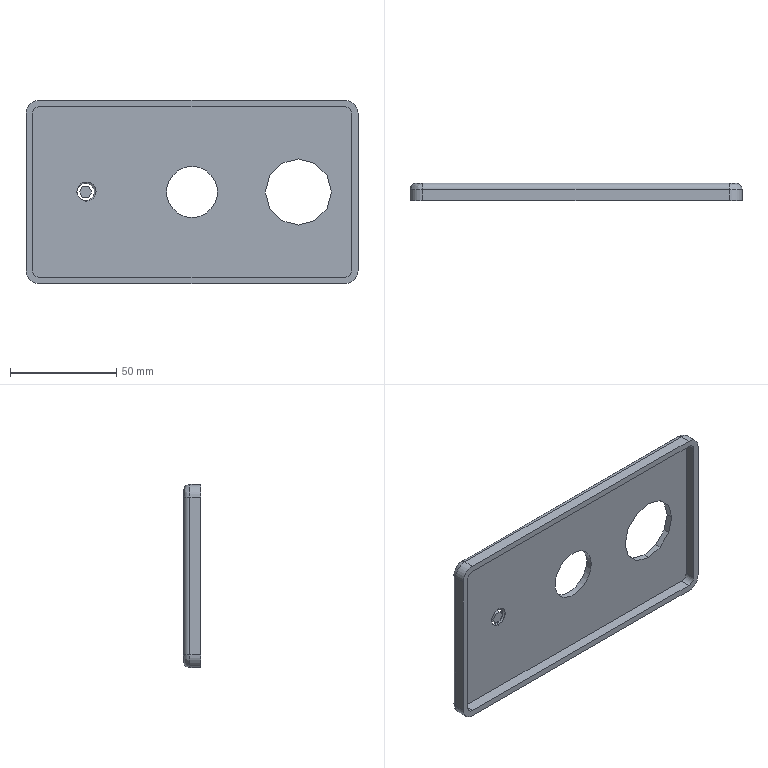Part | SolidWorks | features BaseBody 2 | 2 solids | 61 faces | box 156 x 8 x 86 mm | volume 42531 mm3 | plane 32 | cylinder 23 | spline 6 | commonest cylinder face diameters 6 x8 9.85 x4 12 x4 8.141 x3 10.85 x2 24 x2